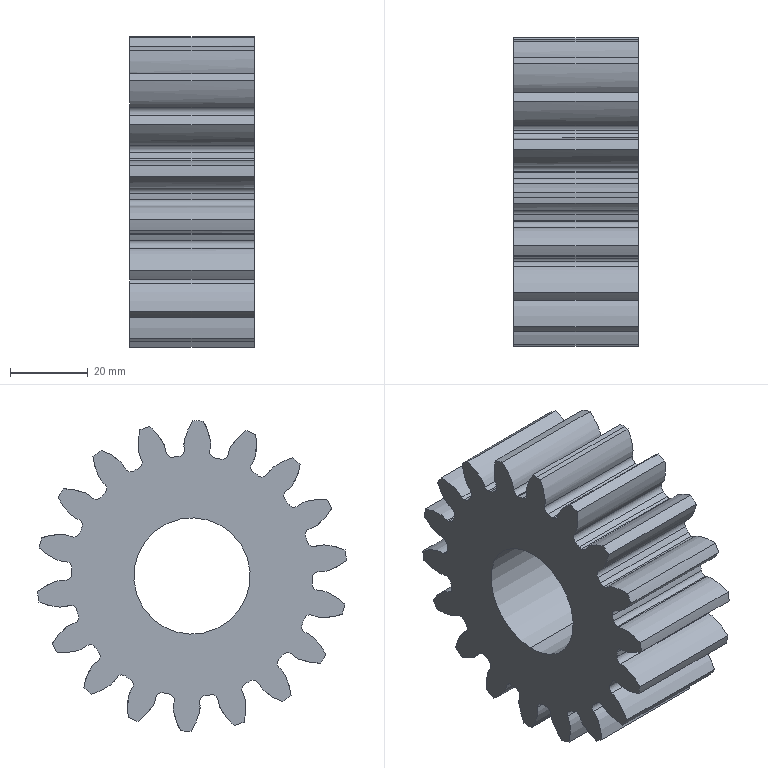Part | NX | features BREP 1 | 1 solid | 121 faces | box 32 x 79.596 x 79.999 mm | volume 104625 mm3 | cylinder 83 | spline 36 | plane 2 | commonest cylinder face diameters 3.04 x44 80 x19 62 x18 30 x2